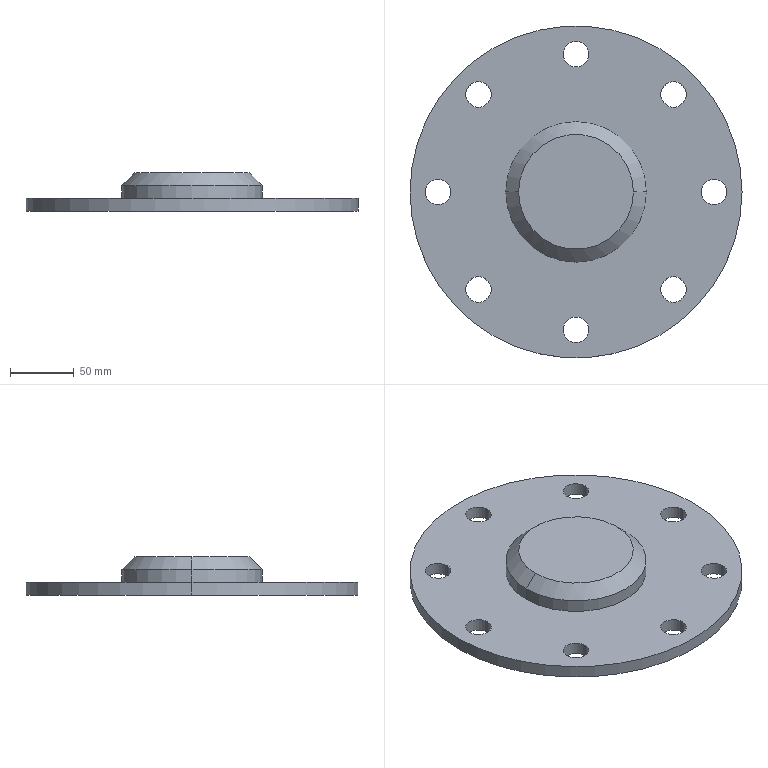Part | SolidWorks | features ICE 2, Chamfer 1, Extrusion 1 | 1 solid | 28 faces | box 260 x 260 x 30 mm | volume 552397 mm3 | cylinder 22 | plane 4 | cone 2 | commonest cylinder face diameters 20 x16 90 x2 110 x2 260 x2
STEP:
#1=CARTESIAN_POINT('',(45.,0.,30.));
#2=VERTEX_POINT('',#1);
#3=CARTESIAN_POINT('',(-45.,0.,30.));
#4=VERTEX_POINT('',#3);
#5=CARTESIAN_POINT('',(0.,0.,30.));
#6=DIRECTION('',(0.,0.,1.));
#7=DIRECTION('',(1.,0.,0.));
#8=AXIS2_PLACEMENT_3D('',#5,#6,#7);
#9=CIRCLE('',#8,45.);
#10=EDGE_CURVE('',#2,#4,#9,.T.);
#11=ORIENTED_EDGE('',*,*,#10,.F.);
#12=CARTESIAN_POINT('',(55.,0.,20.));
#13=VERTEX_POINT('',#12);
#14=CARTESIAN_POINT('',(45.,0.,30.));
#15=DIRECTION('',(0.7071,0.,-0.7071));
#16=VECTOR('',#15,1000.);
#17=LINE('',#14,#16);
#18=EDGE_CURVE('',#2,#13,#17,.T.);
#19=ORIENTED_EDGE('',*,*,#18,.T.);
#20=CARTESIAN_POINT('',(-55.,0.,20.));
#21=VERTEX_POINT('',#20);
#22=CARTESIAN_POINT('',(0.,0.,20.));
#23=DIRECTION('',(0.,0.,-1.));
#24=DIRECTION('',(1.,0.,0.));
#25=AXIS2_PLACEMENT_3D('',#22,#23,#24);
#26=CIRCLE('',#25,55.);
#27=EDGE_CURVE('',#21,#13,#26,.T.);
#28=ORIENTED_EDGE('',*,*,#27,.F.);
#29=CARTESIAN_POINT('',(-45.,0.,30.));
#30=DIRECTION('',(-0.7071,0.,-0.7071));
#31=VECTOR('',#30,1000.);
#32=LINE('',#29,#31);
#33=EDGE_CURVE('',#4,#21,#32,.T.);
#34=ORIENTED_EDGE('',*,*,#33,.F.);
#35=EDGE_LOOP('',(#11,#19,#28,#34));
#36=FACE_OUTER_BOUND('',#35,.T.);
#37=CARTESIAN_POINT('',(0.,0.,30.));
#38=DIRECTION('',(0.,0.,-1.));
#39=DIRECTION('',(-1.,0.,0.));
#40=AXIS2_PLACEMENT_3D('',#37,#38,#39);
#41=CONICAL_SURFACE('',#40,45.,0.7854);
#42=ADVANCED_FACE('',(#36),#41,.T.);
#43=CARTESIAN_POINT('',(45.,0.,20.));
#44=VERTEX_POINT('',#43);
#45=CARTESIAN_POINT('',(-45.,0.,20.));
#46=VERTEX_POINT('',#45);
#47=CARTESIAN_POINT('',(0.,0.,20.));
#48=DIRECTION('',(0.,0.,-1.));
#49=DIRECTION('',(-1.,0.,0.));
#50=AXIS2_PLACEMENT_3D('',#47,#48,#49);
#51=CIRCLE('',#50,45.);
#52=EDGE_CURVE('',#44,#46,#51,.T.);
#53=ORIENTED_EDGE('',*,*,#52,.F.);
#54=CARTESIAN_POINT('',(45.,0.,0.));
#55=VERTEX_POINT('',#54);
#56=CARTESIAN_POINT('',(45.,0.,20.));
#57=DIRECTION('',(0.,0.,-1.));
#58=VECTOR('',#57,1000.);
#59=LINE('',#56,#58);
#60=EDGE_CURVE('',#44,#55,#59,.T.);
#61=ORIENTED_EDGE('',*,*,#60,.T.);
#62=CARTESIAN_POINT('',(-45.,0.,0.));
#63=VERTEX_POINT('',#62);
#64=CARTESIAN_POINT('',(0.,0.,0.));
#65=DIRECTION('',(0.,0.,-1.));
#66=DIRECTION('',(-1.,0.,0.));
#67=AXIS2_PLACEMENT_3D('',#64,#65,#66);
#68=CIRCLE('',#67,45.);
#69=EDGE_CURVE('',#55,#63,#68,.T.);
#70=ORIENTED_EDGE('',*,*,#69,.T.);
#71=CARTESIAN_POINT('',(-45.,0.,20.));
#72=DIRECTION('',(0.,0.,-1.));
#73=VECTOR('',#72,1000.);
#74=LINE('',#71,#73);
#75=EDGE_CURVE('',#46,#63,#74,.T.);
#76=ORIENTED_EDGE('',*,*,#75,.F.);
#77=EDGE_LOOP('',(#53,#61,#70,#76));
#78=FACE_OUTER_BOUND('',#77,.T.);
#79=CARTESIAN_POINT('',(0.,0.,20.));
#80=DIRECTION('',(0.,0.,-1.));
#81=DIRECTION('',(-1.,0.,0.));
#82=AXIS2_PLACEMENT_3D('',#79,#80,#81);
#83=CYLINDRICAL_SURFACE('',#82,45.);
#84=ADVANCED_FACE('',(#78),#83,.F.);
#85=ORIENTED_EDGE('',*,*,#27,.T.);
#86=CARTESIAN_POINT('',(55.,0.,10.));
#87=VERTEX_POINT('',#86);
#88=CARTESIAN_POINT('',(55.,0.,30.));
#89=DIRECTION('',(0.,0.,-1.));
#90=VECTOR('',#89,1000.);
#91=LINE('',#88,#90);
#92=EDGE_CURVE('',#13,#87,#91,.T.);
#93=ORIENTED_EDGE('',*,*,#92,.T.);
#94=CARTESIAN_POINT('',(-55.,0.,10.));
#95=VERTEX_POINT('',#94);
#96=CARTESIAN_POINT('',(0.,0.,10.));
#97=DIRECTION('',(0.,0.,1.));
#98=DIRECTION('',(1.,0.,0.));
#99=AXIS2_PLACEMENT_3D('',#96,#97,#98);
#100=CIRCLE('',#99,55.);
#101=EDGE_CURVE('',#87,#95,#100,.T.);
#102=ORIENTED_EDGE('',*,*,#101,.T.);
#103=CARTESIAN_POINT('',(-55.,0.,30.));
#104=DIRECTION('',(0.,0.,-1.));
#105=VECTOR('',#104,1000.);
#106=LINE('',#103,#105);
#107=EDGE_CURVE('',#21,#95,#106,.T.);
#108=ORIENTED_EDGE('',*,*,#107,.F.);
#109=EDGE_LOOP('',(#85,#93,#102,#108));
#110=FACE_OUTER_BOUND('',#109,.T.);
#111=CARTESIAN_POINT('',(0.,0.,30.));
#112=DIRECTION('',(0.,0.,-1.));
#113=DIRECTION('',(-1.,0.,0.));
#114=AXIS2_PLACEMENT_3D('',#111,#112,#113);
#115=CYLINDRICAL_SURFACE('',#114,55.);
#116=ADVANCED_FACE('',(#110),#115,.T.);
#117=CARTESIAN_POINT('',(-86.368,76.368,10.));
#118=VERTEX_POINT('',#117);
#119=CARTESIAN_POINT('',(-66.368,76.368,10.));
#120=VERTEX_POINT('',#119);
#121=CARTESIAN_POINT('',(-76.368,76.368,10.));
#122=DIRECTION('',(0.,0.,1.));
#123=DIRECTION('',(1.,0.,0.));
#124=AXIS2_PLACEMENT_3D('',#121,#122,#123);
#125=CIRCLE('',#124,10.);
#126=EDGE_CURVE('',#118,#120,#125,.T.);
#127=ORIENTED_EDGE('',*,*,#126,.T.);
#128=CARTESIAN_POINT('',(-66.368,76.368,0.));
#129=VERTEX_POINT('',#128);
#130=CARTESIAN_POINT('',(-66.368,76.368,10.));
#131=DIRECTION('',(0.,0.,-1.));
#132=VECTOR('',#131,1000.);
#133=LINE('',#130,#132);
#134=EDGE_CURVE('',#120,#129,#133,.T.);
#135=ORIENTED_EDGE('',*,*,#134,.T.);
#136=CARTESIAN_POINT('',(-86.368,76.368,0.));
#137=VERTEX_POINT('',#136);
#138=CARTESIAN_POINT('',(-76.368,76.368,0.));
#139=DIRECTION('',(0.,0.,1.));
#140=DIRECTION('',(1.,0.,0.));
#141=AXIS2_PLACEMENT_3D('',#138,#139,#140);
#142=CIRCLE('',#141,10.);
#143=EDGE_CURVE('',#137,#129,#142,.T.);
#144=ORIENTED_EDGE('',*,*,#143,.F.);
#145=CARTESIAN_POINT('',(-86.368,76.368,10.));
#146=DIRECTION('',(0.,0.,-1.));
#147=VECTOR('',#146,1000.);
#148=LINE('',#145,#147);
#149=EDGE_CURVE('',#118,#137,#148,.T.);
#150=ORIENTED_EDGE('',*,*,#149,.F.);
#151=EDGE_LOOP('',(#127,#135,#144,#150));
#152=FACE_OUTER_BOUND('',#151,.T.);
#153=CARTESIAN_POINT('',(-76.368,76.368,10.));
#154=DIRECTION('',(0.,0.,-1.));
#155=DIRECTION('',(-1.,0.,0.));
#156=AXIS2_PLACEMENT_3D('',#153,#154,#155);
#157=CYLINDRICAL_SURFACE('',#156,10.);
#158=ADVANCED_FACE('',(#152),#157,.F.);
#159=CARTESIAN_POINT('',(-118.,0.,10.));
#160=VERTEX_POINT('',#159);
#161=CARTESIAN_POINT('',(-98.,0.,10.));
#162=VERTEX_POINT('',#161);
#163=CARTESIAN_POINT('',(-108.,0.,10.));
#164=DIRECTION('',(0.,0.,1.));
#165=DIRECTION('',(1.,0.,0.));
#166=AXIS2_PLACEMENT_3D('',#163,#164,#165);
#167=CIRCLE('',#166,10.);
#168=EDGE_CURVE('',#160,#162,#167,.T.);
#169=ORIENTED_EDGE('',*,*,#168,.T.);
#170=CARTESIAN_POINT('',(-98.,0.,0.));
#171=VERTEX_POINT('',#170);
#172=CARTESIAN_POINT('',(-98.,0.,10.));
#173=DIRECTION('',(0.,0.,-1.));
#174=VECTOR('',#173,1000.);
#175=LINE('',#172,#174);
#176=EDGE_CURVE('',#162,#171,#175,.T.);
#177=ORIENTED_EDGE('',*,*,#176,.T.);
#178=CARTESIAN_POINT('',(-118.,0.,0.));
#179=VERTEX_POINT('',#178);
#180=CARTESIAN_POINT('',(-108.,0.,0.));
#181=DIRECTION('',(0.,0.,1.));
#182=DIRECTION('',(1.,0.,0.));
#183=AXIS2_PLACEMENT_3D('',#180,#181,#182);
#184=CIRCLE('',#183,10.);
#185=EDGE_CURVE('',#179,#171,#184,.T.);
#186=ORIENTED_EDGE('',*,*,#185,.F.);
#187=CARTESIAN_POINT('',(-118.,0.,10.));
#188=DIRECTION('',(0.,0.,-1.));
#189=VECTOR('',#188,1000.);
#190=LINE('',#187,#189);
#191=EDGE_CURVE('',#160,#179,#190,.T.);
#192=ORIENTED_EDGE('',*,*,#191,.F.);
#193=EDGE_LOOP('',(#169,#177,#186,#192));
#194=FACE_OUTER_BOUND('',#193,.T.);
#195=CARTESIAN_POINT('',(-108.,0.,10.));
#196=DIRECTION('',(0.,0.,-1.));
#197=DIRECTION('',(-1.,0.,0.));
#198=AXIS2_PLACEMENT_3D('',#195,#196,#197);
#199=CYLINDRICAL_SURFACE('',#198,10.);
#200=ADVANCED_FACE('',(#194),#199,.F.);
#201=CARTESIAN_POINT('',(-86.368,-76.368,10.));
#202=VERTEX_POINT('',#201);
#203=CARTESIAN_POINT('',(-66.368,-76.368,10.));
#204=VERTEX_POINT('',#203);
#205=CARTESIAN_POINT('',(-76.368,-76.368,10.));
#206=DIRECTION('',(0.,0.,1.));
#207=DIRECTION('',(1.,0.,0.));
#208=AXIS2_PLACEMENT_3D('',#205,#206,#207);
#209=CIRCLE('',#208,10.);
#210=EDGE_CURVE('',#202,#204,#209,.T.);
#211=ORIENTED_EDGE('',*,*,#210,.T.);
#212=CARTESIAN_POINT('',(-66.368,-76.368,0.));
#213=VERTEX_POINT('',#212);
#214=CARTESIAN_POINT('',(-66.368,-76.368,10.));
#215=DIRECTION('',(0.,0.,-1.));
#216=VECTOR('',#215,1000.);
#217=LINE('',#214,#216);
#218=EDGE_CURVE('',#204,#213,#217,.T.);
#219=ORIENTED_EDGE('',*,*,#218,.T.);
#220=CARTESIAN_POINT('',(-86.368,-76.368,0.));
#221=VERTEX_POINT('',#220);
#222=CARTESIAN_POINT('',(-76.368,-76.368,0.));
#223=DIRECTION('',(0.,0.,1.));
#224=DIRECTION('',(1.,0.,0.));
#225=AXIS2_PLACEMENT_3D('',#222,#223,#224);
#226=CIRCLE('',#225,10.);
#227=EDGE_CURVE('',#221,#213,#226,.T.);
#228=ORIENTED_EDGE('',*,*,#227,.F.);
#229=CARTESIAN_POINT('',(-86.368,-76.368,10.));
#230=DIRECTION('',(0.,0.,-1.));
#231=VECTOR('',#230,1000.);
#232=LINE('',#229,#231);
#233=EDGE_CURVE('',#202,#221,#232,.T.);
#234=ORIENTED_EDGE('',*,*,#233,.F.);
#235=EDGE_LOOP('',(#211,#219,#228,#234));
#236=FACE_OUTER_BOUND('',#235,.T.);
#237=CARTESIAN_POINT('',(-76.368,-76.368,10.));
#238=DIRECTION('',(0.,0.,-1.));
#239=DIRECTION('',(-1.,0.,0.));
#240=AXIS2_PLACEMENT_3D('',#237,#238,#239);
#241=CYLINDRICAL_SURFACE('',#240,10.);
#242=ADVANCED_FACE('',(#236),#241,.F.);
#243=CARTESIAN_POINT('',(-10.,-108.,10.));
#244=VERTEX_POINT('',#243);
#245=CARTESIAN_POINT('',(10.,-108.,10.));
#246=VERTEX_POINT('',#245);
#247=CARTESIAN_POINT('',(0.,-108.,10.));
#248=DIRECTION('',(0.,0.,1.));
#249=DIRECTION('',(1.,0.,0.));
#250=AXIS2_PLACEMENT_3D('',#247,#248,#249);
#251=CIRCLE('',#250,10.);
#252=EDGE_CURVE('',#244,#246,#251,.T.);
#253=ORIENTED_EDGE('',*,*,#252,.T.);
#254=CARTESIAN_POINT('',(10.,-108.,0.));
#255=VERTEX_POINT('',#254);
#256=CARTESIAN_POINT('',(10.,-108.,10.));
#257=DIRECTION('',(0.,0.,-1.));
#258=VECTOR('',#257,1000.);
#259=LINE('',#256,#258);
#260=EDGE_CURVE('',#246,#255,#259,.T.);
#261=ORIENTED_EDGE('',*,*,#260,.T.);
#262=CARTESIAN_POINT('',(-10.,-108.,0.));
#263=VERTEX_POINT('',#262);
#264=CARTESIAN_POINT('',(0.,-108.,0.));
#265=DIRECTION('',(0.,0.,1.));
#266=DIRECTION('',(1.,0.,0.));
#267=AXIS2_PLACEMENT_3D('',#264,#265,#266);
#268=CIRCLE('',#267,10.);
#269=EDGE_CURVE('',#263,#255,#268,.T.);
#270=ORIENTED_EDGE('',*,*,#269,.F.);
#271=CARTESIAN_POINT('',(-10.,-108.,10.));
#272=DIRECTION('',(0.,0.,-1.));
#273=VECTOR('',#272,1000.);
#274=LINE('',#271,#273);
#275=EDGE_CURVE('',#244,#263,#274,.T.);
#276=ORIENTED_EDGE('',*,*,#275,.F.);
#277=EDGE_LOOP('',(#253,#261,#270,#276));
#278=FACE_OUTER_BOUND('',#277,.T.);
#279=CARTESIAN_POINT('',(0.,-108.,10.));
#280=DIRECTION('',(0.,0.,-1.));
#281=DIRECTION('',(-1.,0.,0.));
#282=AXIS2_PLACEMENT_3D('',#279,#280,#281);
#283=CYLINDRICAL_SURFACE('',#282,10.);
#284=ADVANCED_FACE('',(#278),#283,.F.);
#285=CARTESIAN_POINT('',(66.368,-76.368,10.));
#286=VERTEX_POINT('',#285);
#287=CARTESIAN_POINT('',(86.368,-76.368,10.));
#288=VERTEX_POINT('',#287);
#289=CARTESIAN_POINT('',(76.368,-76.368,10.));
#290=DIRECTION('',(0.,0.,1.));
#291=DIRECTION('',(1.,0.,0.));
#292=AXIS2_PLACEMENT_3D('',#289,#290,#291);
#293=CIRCLE('',#292,10.);
#294=EDGE_CURVE('',#286,#288,#293,.T.);
#295=ORIENTED_EDGE('',*,*,#294,.T.);
#296=CARTESIAN_POINT('',(86.368,-76.368,0.));
#297=VERTEX_POINT('',#296);
#298=CARTESIAN_POINT('',(86.368,-76.368,10.));
#299=DIRECTION('',(0.,0.,-1.));
#300=VECTOR('',#299,1000.);
#301=LINE('',#298,#300);
#302=EDGE_CURVE('',#288,#297,#301,.T.);
#303=ORIENTED_EDGE('',*,*,#302,.T.);
#304=CARTESIAN_POINT('',(66.368,-76.368,0.));
#305=VERTEX_POINT('',#304);
#306=CARTESIAN_POINT('',(76.368,-76.368,0.));
#307=DIRECTION('',(0.,0.,1.));
#308=DIRECTION('',(1.,0.,0.));
#309=AXIS2_PLACEMENT_3D('',#306,#307,#308);
#310=CIRCLE('',#309,10.);
#311=EDGE_CURVE('',#305,#297,#310,.T.);
#312=ORIENTED_EDGE('',*,*,#311,.F.);
#313=CARTESIAN_POINT('',(66.368,-76.368,10.));
#314=DIRECTION('',(0.,0.,-1.));
#315=VECTOR('',#314,1000.);
#316=LINE('',#313,#315);
#317=EDGE_CURVE('',#286,#305,#316,.T.);
#318=ORIENTED_EDGE('',*,*,#317,.F.);
#319=EDGE_LOOP('',(#295,#303,#312,#318));
#320=FACE_OUTER_BOUND('',#319,.T.);
#321=CARTESIAN_POINT('',(76.368,-76.368,10.));
#322=DIRECTION('',(0.,0.,-1.));
#323=DIRECTION('',(-1.,0.,0.));
#324=AXIS2_PLACEMENT_3D('',#321,#322,#323);
#325=CYLINDRICAL_SURFACE('',#324,10.);
#326=ADVANCED_FACE('',(#320),#325,.F.);
#327=CARTESIAN_POINT('',(98.,0.,10.));
#328=VERTEX_POINT('',#327);
#329=CARTESIAN_POINT('',(118.,0.,10.));
#330=VERTEX_POINT('',#329);
#331=CARTESIAN_POINT('',(108.,0.,10.));
#332=DIRECTION('',(0.,0.,1.));
#333=DIRECTION('',(1.,0.,0.));
#334=AXIS2_PLACEMENT_3D('',#331,#332,#333);
#335=CIRCLE('',#334,10.);
#336=EDGE_CURVE('',#328,#330,#335,.T.);
#337=ORIENTED_EDGE('',*,*,#336,.T.);
#338=CARTESIAN_POINT('',(118.,0.,0.));
#339=VERTEX_POINT('',#338);
#340=CARTESIAN_POINT('',(118.,0.,10.));
#341=DIRECTION('',(0.,0.,-1.));
#342=VECTOR('',#341,1000.);
#343=LINE('',#340,#342);
#344=EDGE_CURVE('',#330,#339,#343,.T.);
#345=ORIENTED_EDGE('',*,*,#344,.T.);
#346=CARTESIAN_POINT('',(98.,0.,0.));
#347=VERTEX_POINT('',#346);
#348=CARTESIAN_POINT('',(108.,0.,0.));
#349=DIRECTION('',(0.,0.,1.));
#350=DIRECTION('',(1.,0.,0.));
#351=AXIS2_PLACEMENT_3D('',#348,#349,#350);
#352=CIRCLE('',#351,10.);
#353=EDGE_CURVE('',#347,#339,#352,.T.);
#354=ORIENTED_EDGE('',*,*,#353,.F.);
#355=CARTESIAN_POINT('',(98.,0.,10.));
#356=DIRECTION('',(0.,0.,-1.));
#357=VECTOR('',#356,1000.);
#358=LINE('',#355,#357);
#359=EDGE_CURVE('',#328,#347,#358,.T.);
#360=ORIENTED_EDGE('',*,*,#359,.F.);
#361=EDGE_LOOP('',(#337,#345,#354,#360));
#362=FACE_OUTER_BOUND('',#361,.T.);
#363=CARTESIAN_POINT('',(108.,0.,10.));
#364=DIRECTION('',(0.,0.,-1.));
#365=DIRECTION('',(-1.,0.,0.));
#366=AXIS2_PLACEMENT_3D('',#363,#364,#365);
#367=CYLINDRICAL_SURFACE('',#366,10.);
#368=ADVANCED_FACE('',(#362),#367,.F.);
#369=CARTESIAN_POINT('',(66.368,76.368,10.));
#370=VERTEX_POINT('',#369);
#371=CARTESIAN_POINT('',(86.368,76.368,10.));
#372=VERTEX_POINT('',#371);
#373=CARTESIAN_POINT('',(76.368,76.368,10.));
#374=DIRECTION('',(0.,0.,1.));
#375=DIRECTION('',(1.,0.,0.));
#376=AXIS2_PLACEMENT_3D('',#373,#374,#375);
#377=CIRCLE('',#376,10.);
#378=EDGE_CURVE('',#370,#372,#377,.T.);
#379=ORIENTED_EDGE('',*,*,#378,.T.);
#380=CARTESIAN_POINT('',(86.368,76.368,0.));
#381=VERTEX_POINT('',#380);
#382=CARTESIAN_POINT('',(86.368,76.368,10.));
#383=DIRECTION('',(0.,0.,-1.));
#384=VECTOR('',#383,1000.);
#385=LINE('',#382,#384);
#386=EDGE_CURVE('',#372,#381,#385,.T.);
#387=ORIENTED_EDGE('',*,*,#386,.T.);
#388=CARTESIAN_POINT('',(66.368,76.368,0.));
#389=VERTEX_POINT('',#388);
#390=CARTESIAN_POINT('',(76.368,76.368,0.));
#391=DIRECTION('',(0.,0.,1.));
#392=DIRECTION('',(1.,0.,0.));
#393=AXIS2_PLACEMENT_3D('',#390,#391,#392);
#394=CIRCLE('',#393,10.);
#395=EDGE_CURVE('',#389,#381,#394,.T.);
#396=ORIENTED_EDGE('',*,*,#395,.F.);
#397=CARTESIAN_POINT('',(66.368,76.368,10.));
#398=DIRECTION('',(0.,0.,-1.));
#399=VECTOR('',#398,1000.);
#400=LINE('',#397,#399);
#401=EDGE_CURVE('',#370,#389,#400,.T.);
#402=ORIENTED_EDGE('',*,*,#401,.F.);
#403=EDGE_LOOP('',(#379,#387,#396,#402));
#404=FACE_OUTER_BOUND('',#403,.T.);
#405=CARTESIAN_POINT('',(76.368,76.368,10.));
#406=DIRECTION('',(0.,0.,-1.));
#407=DIRECTION('',(-1.,0.,0.));
#408=AXIS2_PLACEMENT_3D('',#405,#406,#407);
#409=CYLINDRICAL_SURFACE('',#408,10.);
#410=ADVANCED_FACE('',(#404),#409,.F.);
#411=CARTESIAN_POINT('',(-10.,108.,10.));
#412=VERTEX_POINT('',#411);
#413=CARTESIAN_POINT('',(10.,108.,10.));
#414=VERTEX_POINT('',#413);
#415=CARTESIAN_POINT('',(0.,108.,10.));
#416=DIRECTION('',(0.,0.,1.));
#417=DIRECTION('',(1.,0.,0.));
#418=AXIS2_PLACEMENT_3D('',#415,#416,#417);
#419=CIRCLE('',#418,10.);
#420=EDGE_CURVE('',#412,#414,#419,.T.);
#421=ORIENTED_EDGE('',*,*,#420,.T.);
#422=CARTESIAN_POINT('',(10.,108.,0.));
#423=VERTEX_POINT('',#422);
#424=CARTESIAN_POINT('',(10.,108.,10.));
#425=DIRECTION('',(0.,0.,-1.));
#426=VECTOR('',#425,1000.);
#427=LINE('',#424,#426);
#428=EDGE_CURVE('',#414,#423,#427,.T.);
#429=ORIENTED_EDGE('',*,*,#428,.T.);
#430=CARTESIAN_POINT('',(-10.,108.,0.));
#431=VERTEX_POINT('',#430);
#432=CARTESIAN_POINT('',(0.,108.,0.));
#433=DIRECTION('',(0.,0.,1.));
#434=DIRECTION('',(1.,0.,0.));
#435=AXIS2_PLACEMENT_3D('',#432,#433,#434);
#436=CIRCLE('',#435,10.);
#437=EDGE_CURVE('',#431,#423,#436,.T.);
#438=ORIENTED_EDGE('',*,*,#437,.F.);
#439=CARTESIAN_POINT('',(-10.,108.,10.));
#440=DIRECTION('',(0.,0.,-1.));
#441=VECTOR('',#440,1000.);
#442=LINE('',#439,#441);
#443=EDGE_CURVE('',#412,#431,#442,.T.);
#444=ORIENTED_EDGE('',*,*,#443,.F.);
#445=EDGE_LOOP('',(#421,#429,#438,#444));
#446=FACE_OUTER_BOUND('',#445,.T.);
#447=CARTESIAN_POINT('',(0.,108.,10.));
#448=DIRECTION('',(0.,0.,-1.));
#449=DIRECTION('',(-1.,0.,0.));
#450=AXIS2_PLACEMENT_3D('',#447,#448,#449);
#451=CYLINDRICAL_SURFACE('',#450,10.);
#452=ADVANCED_FACE('',(#446),#451,.F.);
#453=CARTESIAN_POINT('',(130.,0.,10.));
#454=VERTEX_POINT('',#453);
#455=CARTESIAN_POINT('',(-130.,0.,10.));
#456=VERTEX_POINT('',#455);
#457=CARTESIAN_POINT('',(0.,0.,10.));
#458=DIRECTION('',(0.,0.,1.));
#459=DIRECTION('',(1.,0.,0.));
#460=AXIS2_PLACEMENT_3D('',#457,#458,#459);
#461=CIRCLE('',#460,130.);
#462=EDGE_CURVE('',#454,#456,#461,.T.);
#463=ORIENTED_EDGE('',*,*,#462,.F.);
#464=CARTESIAN_POINT('',(130.,0.,0.));
#465=VERTEX_POINT('',#464);
#466=CARTESIAN_POINT('',(130.,0.,10.));
#467=DIRECTION('',(0.,0.,-1.));
#468=VECTOR('',#467,1000.);
#469=LINE('',#466,#468);
#470=EDGE_CURVE('',#454,#465,#469,.T.);
#471=ORIENTED_EDGE('',*,*,#470,.T.);
#472=CARTESIAN_POINT('',(-130.,0.,0.));
#473=VERTEX_POINT('',#472);
#474=CARTESIAN_POINT('',(0.,0.,0.));
#475=DIRECTION('',(0.,0.,1.));
#476=DIRECTION('',(1.,0.,0.));
#477=AXIS2_PLACEMENT_3D('',#474,#475,#476);
#478=CIRCLE('',#477,130.);
#479=EDGE_CURVE('',#465,#473,#478,.T.);
#480=ORIENTED_EDGE('',*,*,#479,.T.);
#481=CARTESIAN_POINT('',(-130.,0.,10.));
#482=DIRECTION('',(0.,0.,-1.));
#483=VECTOR('',#482,1000.);
#484=LINE('',#481,#483);
#485=EDGE_CURVE('',#456,#473,#484,.T.);
#486=ORIENTED_EDGE('',*,*,#485,.F.);
#487=EDGE_LOOP('',(#463,#471,#480,#486));
#488=FACE_OUTER_BOUND('',#487,.T.);
#489=CARTESIAN_POINT('',(0.,0.,10.));
#490=DIRECTION('',(0.,0.,-1.));
#491=DIRECTION('',(-1.,0.,0.));
#492=AXIS2_PLACEMENT_3D('',#489,#490,#491);
#493=CYLINDRICAL_SURFACE('',#492,130.);
#494=ADVANCED_FACE('',(#488),#493,.T.);
#495=CARTESIAN_POINT('',(0.,0.,10.));
#496=DIRECTION('',(0.,0.,1.));
#497=DIRECTION('',(1.,0.,0.));
#498=AXIS2_PLACEMENT_3D('',#495,#496,#497);
#499=CIRCLE('',#498,55.);
#500=EDGE_CURVE('',#95,#87,#499,.T.);
#501=ORIENTED_EDGE('',*,*,#500,.F.);
#502=ORIENTED_EDGE('',*,*,#101,.F.);
#503=EDGE_LOOP('',(#501,#502));
#504=FACE_BOUND('',#503,.T.);
#505=ORIENTED_EDGE('',*,*,#168,.F.);
#506=CARTESIAN_POINT('',(-108.,0.,10.));
#507=DIRECTION('',(0.,0.,1.));
#508=DIRECTION('',(1.,0.,0.));
#509=AXIS2_PLACEMENT_3D('',#506,#507,#508);
#510=CIRCLE('',#509,10.);
#511=EDGE_CURVE('',#162,#160,#510,.T.);
#512=ORIENTED_EDGE('',*,*,#511,.F.);
#513=EDGE_LOOP('',(#505,#512));
#514=FACE_BOUND('',#513,.T.);
#515=ORIENTED_EDGE('',*,*,#252,.F.);
#516=CARTESIAN_POINT('',(0.,-108.,10.));
#517=DIRECTION('',(0.,0.,1.));
#518=DIRECTION('',(1.,0.,0.));
#519=AXIS2_PLACEMENT_3D('',#516,#517,#518);
#520=CIRCLE('',#519,10.);
#521=EDGE_CURVE('',#246,#244,#520,.T.);
#522=ORIENTED_EDGE('',*,*,#521,.F.);
#523=EDGE_LOOP('',(#515,#522));
#524=FACE_BOUND('',#523,.T.);
#525=ORIENTED_EDGE('',*,*,#336,.F.);
#526=CARTESIAN_POINT('',(108.,0.,10.));
#527=DIRECTION('',(0.,0.,1.));
#528=DIRECTION('',(1.,0.,0.));
#529=AXIS2_PLACEMENT_3D('',#526,#527,#528);
#530=CIRCLE('',#529,10.);
#531=EDGE_CURVE('',#330,#328,#530,.T.);
#532=ORIENTED_EDGE('',*,*,#531,.F.);
#533=EDGE_LOOP('',(#525,#532));
#534=FACE_BOUND('',#533,.T.);
#535=ORIENTED_EDGE('',*,*,#420,.F.);
#536=CARTESIAN_POINT('',(0.,108.,10.));
#537=DIRECTION('',(0.,0.,1.));
#538=DIRECTION('',(1.,0.,0.));
#539=AXIS2_PLACEMENT_3D('',#536,#537,#538);
#540=CIRCLE('',#539,10.);
#541=EDGE_CURVE('',#414,#412,#540,.T.);
#542=ORIENTED_EDGE('',*,*,#541,.F.);
#543=EDGE_LOOP('',(#535,#542));
#544=FACE_BOUND('',#543,.T.);
#545=CARTESIAN_POINT('',(0.,0.,10.));
#546=DIRECTION('',(0.,0.,1.));
#547=DIRECTION('',(1.,0.,0.));
#548=AXIS2_PLACEMENT_3D('',#545,#546,#547);
#549=CIRCLE('',#548,130.);
#550=EDGE_CURVE('',#456,#454,#549,.T.);
#551=ORIENTED_EDGE('',*,*,#550,.T.);
#552=ORIENTED_EDGE('',*,*,#462,.T.);
#553=EDGE_LOOP('',(#551,#552));
#554=FACE_OUTER_BOUND('',#553,.T.);
#555=ORIENTED_EDGE('',*,*,#378,.F.);
#556=CARTESIAN_POINT('',(76.368,76.368,10.));
#557=DIRECTION('',(0.,0.,1.));
#558=DIRECTION('',(1.,0.,0.));
#559=AXIS2_PLACEMENT_3D('',#556,#557,#558);
#560=CIRCLE('',#559,10.);
#561=EDGE_CURVE('',#372,#370,#560,.T.);
#562=ORIENTED_EDGE('',*,*,#561,.F.);
#563=EDGE_LOOP('',(#555,#562));
#564=FACE_BOUND('',#563,.T.);
#565=ORIENTED_EDGE('',*,*,#294,.F.);
#566=CARTESIAN_POINT('',(76.368,-76.368,10.));
#567=DIRECTION('',(0.,0.,1.));
#568=DIRECTION('',(1.,0.,0.));
#569=AXIS2_PLACEMENT_3D('',#566,#567,#568);
#570=CIRCLE('',#569,10.);
#571=EDGE_CURVE('',#288,#286,#570,.T.);
#572=ORIENTED_EDGE('',*,*,#571,.F.);
#573=EDGE_LOOP('',(#565,#572));
#574=FACE_BOUND('',#573,.T.);
#575=ORIENTED_EDGE('',*,*,#210,.F.);
#576=CARTESIAN_POINT('',(-76.368,-76.368,10.));
#577=DIRECTION('',(0.,0.,1.));
#578=DIRECTION('',(1.,0.,0.));
#579=AXIS2_PLACEMENT_3D('',#576,#577,#578);
#580=CIRCLE('',#579,10.);
#581=EDGE_CURVE('',#204,#202,#580,.T.);
#582=ORIENTED_EDGE('',*,*,#581,.F.);
#583=EDGE_LOOP('',(#575,#582));
#584=FACE_BOUND('',#583,.T.);
#585=ORIENTED_EDGE('',*,*,#126,.F.);
#586=CARTESIAN_POINT('',(-76.368,76.368,10.));
#587=DIRECTION('',(0.,0.,1.));
#588=DIRECTION('',(1.,0.,0.));
#589=AXIS2_PLACEMENT_3D('',#586,#587,#588);
#590=CIRCLE('',#589,10.);
#591=EDGE_CURVE('',#120,#118,#590,.T.);
#592=ORIENTED_EDGE('',*,*,#591,.F.);
#593=EDGE_LOOP('',(#585,#592));
#594=FACE_BOUND('',#593,.T.);
#595=CARTESIAN_POINT('',(0.,0.,10.));
#596=DIRECTION('',(0.,0.,1.));
#597=DIRECTION('',(1.,0.,0.));
#598=AXIS2_PLACEMENT_3D('',#595,#596,#597);
#599=PLANE('',#598);
#600=ADVANCED_FACE('',(#504,#514,#524,#534,#544,#554,#564,#574,#584,#594),#599,.T.);
#601=CARTESIAN_POINT('',(0.,0.,0.));
#602=DIRECTION('',(0.,0.,-1.));
#603=DIRECTION('',(-1.,0.,0.));
#604=AXIS2_PLACEMENT_3D('',#601,#602,#603);
#605=CIRCLE('',#604,45.);
#606=EDGE_CURVE('',#63,#55,#605,.T.);
#607=ORIENTED_EDGE('',*,*,#606,.F.);
#608=ORIENTED_EDGE('',*,*,#69,.F.);
#609=EDGE_LOOP('',(#607,#608));
#610=FACE_BOUND('',#609,.T.);
#611=CARTESIAN_POINT('',(0.,0.,0.));
#612=DIRECTION('',(0.,0.,1.));
#613=DIRECTION('',(1.,0.,0.));
#614=AXIS2_PLACEMENT_3D('',#611,#612,#613);
#615=CIRCLE('',#614,130.);
#616=EDGE_CURVE('',#473,#465,#615,.T.);
#617=ORIENTED_EDGE('',*,*,#616,.F.);
#618=ORIENTED_EDGE('',*,*,#479,.F.);
#619=EDGE_LOOP('',(#617,#618));
#620=FACE_OUTER_BOUND('',#619,.T.);
#621=ORIENTED_EDGE('',*,*,#437,.T.);
#622=CARTESIAN_POINT('',(0.,108.,0.));
#623=DIRECTION('',(0.,0.,1.));
#624=DIRECTION('',(1.,0.,0.));
#625=AXIS2_PLACEMENT_3D('',#622,#623,#624);
#626=CIRCLE('',#625,10.);
#627=EDGE_CURVE('',#423,#431,#626,.T.);
#628=ORIENTED_EDGE('',*,*,#627,.T.);
#629=EDGE_LOOP('',(#621,#628));
#630=FACE_BOUND('',#629,.T.);
#631=ORIENTED_EDGE('',*,*,#395,.T.);
#632=CARTESIAN_POINT('',(76.368,76.368,0.));
#633=DIRECTION('',(0.,0.,1.));
#634=DIRECTION('',(1.,0.,0.));
#635=AXIS2_PLACEMENT_3D('',#632,#633,#634);
#636=CIRCLE('',#635,10.);
#637=EDGE_CURVE('',#381,#389,#636,.T.);
#638=ORIENTED_EDGE('',*,*,#637,.T.);
#639=EDGE_LOOP('',(#631,#638));
#640=FACE_BOUND('',#639,.T.);
#641=ORIENTED_EDGE('',*,*,#353,.T.);
#642=CARTESIAN_POINT('',(108.,0.,0.));
#643=DIRECTION('',(0.,0.,1.));
#644=DIRECTION('',(1.,0.,0.));
#645=AXIS2_PLACEMENT_3D('',#642,#643,#644);
#646=CIRCLE('',#645,10.);
#647=EDGE_CURVE('',#339,#347,#646,.T.);
#648=ORIENTED_EDGE('',*,*,#647,.T.);
#649=EDGE_LOOP('',(#641,#648));
#650=FACE_BOUND('',#649,.T.);
#651=ORIENTED_EDGE('',*,*,#311,.T.);
#652=CARTESIAN_POINT('',(76.368,-76.368,0.));
#653=DIRECTION('',(0.,0.,1.));
#654=DIRECTION('',(1.,0.,0.));
#655=AXIS2_PLACEMENT_3D('',#652,#653,#654);
#656=CIRCLE('',#655,10.);
#657=EDGE_CURVE('',#297,#305,#656,.T.);
#658=ORIENTED_EDGE('',*,*,#657,.T.);
#659=EDGE_LOOP('',(#651,#658));
#660=FACE_BOUND('',#659,.T.);
#661=ORIENTED_EDGE('',*,*,#269,.T.);
#662=CARTESIAN_POINT('',(0.,-108.,0.));
#663=DIRECTION('',(0.,0.,1.));
#664=DIRECTION('',(1.,0.,0.));
#665=AXIS2_PLACEMENT_3D('',#662,#663,#664);
#666=CIRCLE('',#665,10.);
#667=EDGE_CURVE('',#255,#263,#666,.T.);
#668=ORIENTED_EDGE('',*,*,#667,.T.);
#669=EDGE_LOOP('',(#661,#668));
#670=FACE_BOUND('',#669,.T.);
#671=ORIENTED_EDGE('',*,*,#227,.T.);
#672=CARTESIAN_POINT('',(-76.368,-76.368,0.));
#673=DIRECTION('',(0.,0.,1.));
#674=DIRECTION('',(1.,0.,0.));
#675=AXIS2_PLACEMENT_3D('',#672,#673,#674);
#676=CIRCLE('',#675,10.);
#677=EDGE_CURVE('',#213,#221,#676,.T.);
#678=ORIENTED_EDGE('',*,*,#677,.T.);
#679=EDGE_LOOP('',(#671,#678));
#680=FACE_BOUND('',#679,.T.);
#681=ORIENTED_EDGE('',*,*,#185,.T.);
#682=CARTESIAN_POINT('',(-108.,0.,0.));
#683=DIRECTION('',(0.,0.,1.));
#684=DIRECTION('',(1.,0.,0.));
#685=AXIS2_PLACEMENT_3D('',#682,#683,#684);
#686=CIRCLE('',#685,10.);
#687=EDGE_CURVE('',#171,#179,#686,.T.);
#688=ORIENTED_EDGE('',*,*,#687,.T.);
#689=EDGE_LOOP('',(#681,#688));
#690=FACE_BOUND('',#689,.T.);
#691=ORIENTED_EDGE('',*,*,#143,.T.);
#692=CARTESIAN_POINT('',(-76.368,76.368,0.));
#693=DIRECTION('',(0.,0.,1.));
#694=DIRECTION('',(1.,0.,0.));
#695=AXIS2_PLACEMENT_3D('',#692,#693,#694);
#696=CIRCLE('',#695,10.);
#697=EDGE_CURVE('',#129,#137,#696,.T.);
#698=ORIENTED_EDGE('',*,*,#697,.T.);
#699=EDGE_LOOP('',(#691,#698));
#700=FACE_BOUND('',#699,.T.);
#701=CARTESIAN_POINT('',(0.,0.,0.));
#702=DIRECTION('',(0.,0.,1.));
#703=DIRECTION('',(1.,0.,0.));
#704=AXIS2_PLACEMENT_3D('',#701,#702,#703);
#705=PLANE('',#704);
#706=ADVANCED_FACE('',(#610,#620,#630,#640,#650,#660,#670,#680,#690,#700),#705,.F.);
#707=ORIENTED_EDGE('',*,*,#470,.F.);
#708=ORIENTED_EDGE('',*,*,#550,.F.);
#709=ORIENTED_EDGE('',*,*,#485,.T.);
#710=ORIENTED_EDGE('',*,*,#616,.T.);
#711=EDGE_LOOP('',(#707,#708,#709,#710));
#712=FACE_OUTER_BOUND('',#711,.T.);
#713=CARTESIAN_POINT('',(0.,0.,10.));
#714=DIRECTION('',(0.,0.,-1.));
#715=DIRECTION('',(-1.,0.,0.));
#716=AXIS2_PLACEMENT_3D('',#713,#714,#715);
#717=CYLINDRICAL_SURFACE('',#716,130.);
#718=ADVANCED_FACE('',(#712),#717,.T.);
#719=ORIENTED_EDGE('',*,*,#428,.F.);
#720=ORIENTED_EDGE('',*,*,#541,.T.);
#721=ORIENTED_EDGE('',*,*,#443,.T.);
#722=ORIENTED_EDGE('',*,*,#627,.F.);
#723=EDGE_LOOP('',(#719,#720,#721,#722));
#724=FACE_OUTER_BOUND('',#723,.T.);
#725=CARTESIAN_POINT('',(0.,108.,10.));
#726=DIRECTION('',(0.,0.,-1.));
#727=DIRECTION('',(-1.,0.,0.));
#728=AXIS2_PLACEMENT_3D('',#725,#726,#727);
#729=CYLINDRICAL_SURFACE('',#728,10.);
#730=ADVANCED_FACE('',(#724),#729,.F.);
#731=ORIENTED_EDGE('',*,*,#386,.F.);
#732=ORIENTED_EDGE('',*,*,#561,.T.);
#733=ORIENTED_EDGE('',*,*,#401,.T.);
#734=ORIENTED_EDGE('',*,*,#637,.F.);
#735=EDGE_LOOP('',(#731,#732,#733,#734));
#736=FACE_OUTER_BOUND('',#735,.T.);
#737=CARTESIAN_POINT('',(76.368,76.368,10.));
#738=DIRECTION('',(0.,0.,-1.));
#739=DIRECTION('',(-1.,0.,0.));
#740=AXIS2_PLACEMENT_3D('',#737,#738,#739);
#741=CYLINDRICAL_SURFACE('',#740,10.);
#742=ADVANCED_FACE('',(#736),#741,.F.);
#743=ORIENTED_EDGE('',*,*,#344,.F.);
#744=ORIENTED_EDGE('',*,*,#531,.T.);
#745=ORIENTED_EDGE('',*,*,#359,.T.);
#746=ORIENTED_EDGE('',*,*,#647,.F.);
#747=EDGE_LOOP('',(#743,#744,#745,#746));
#748=FACE_OUTER_BOUND('',#747,.T.);
#749=CARTESIAN_POINT('',(108.,0.,10.));
#750=DIRECTION('',(0.,0.,-1.));
#751=DIRECTION('',(-1.,0.,0.));
#752=AXIS2_PLACEMENT_3D('',#749,#750,#751);
#753=CYLINDRICAL_SURFACE('',#752,10.);
#754=ADVANCED_FACE('',(#748),#753,.F.);
#755=ORIENTED_EDGE('',*,*,#302,.F.);
#756=ORIENTED_EDGE('',*,*,#571,.T.);
#757=ORIENTED_EDGE('',*,*,#317,.T.);
#758=ORIENTED_EDGE('',*,*,#657,.F.);
#759=EDGE_LOOP('',(#755,#756,#757,#758));
#760=FACE_OUTER_BOUND('',#759,.T.);
#761=CARTESIAN_POINT('',(76.368,-76.368,10.));
#762=DIRECTION('',(0.,0.,-1.));
#763=DIRECTION('',(-1.,0.,0.));
#764=AXIS2_PLACEMENT_3D('',#761,#762,#763);
#765=CYLINDRICAL_SURFACE('',#764,10.);
#766=ADVANCED_FACE('',(#760),#765,.F.);
#767=ORIENTED_EDGE('',*,*,#260,.F.);
#768=ORIENTED_EDGE('',*,*,#521,.T.);
#769=ORIENTED_EDGE('',*,*,#275,.T.);
#770=ORIENTED_EDGE('',*,*,#667,.F.);
#771=EDGE_LOOP('',(#767,#768,#769,#770));
#772=FACE_OUTER_BOUND('',#771,.T.);
#773=CARTESIAN_POINT('',(0.,-108.,10.));
#774=DIRECTION('',(0.,0.,-1.));
#775=DIRECTION('',(-1.,0.,0.));
#776=AXIS2_PLACEMENT_3D('',#773,#774,#775);
#777=CYLINDRICAL_SURFACE('',#776,10.);
#778=ADVANCED_FACE('',(#772),#777,.F.);
#779=ORIENTED_EDGE('',*,*,#218,.F.);
#780=ORIENTED_EDGE('',*,*,#581,.T.);
#781=ORIENTED_EDGE('',*,*,#233,.T.);
#782=ORIENTED_EDGE('',*,*,#677,.F.);
#783=EDGE_LOOP('',(#779,#780,#781,#782));
#784=FACE_OUTER_BOUND('',#783,.T.);
#785=CARTESIAN_POINT('',(-76.368,-76.368,10.));
#786=DIRECTION('',(0.,0.,-1.));
#787=DIRECTION('',(-1.,0.,0.));
#788=AXIS2_PLACEMENT_3D('',#785,#786,#787);
#789=CYLINDRICAL_SURFACE('',#788,10.);
#790=ADVANCED_FACE('',(#784),#789,.F.);
#791=ORIENTED_EDGE('',*,*,#176,.F.);
#792=ORIENTED_EDGE('',*,*,#511,.T.);
#793=ORIENTED_EDGE('',*,*,#191,.T.);
#794=ORIENTED_EDGE('',*,*,#687,.F.);
#795=EDGE_LOOP('',(#791,#792,#793,#794));
#796=FACE_OUTER_BOUND('',#795,.T.);
#797=CARTESIAN_POINT('',(-108.,0.,10.));
#798=DIRECTION('',(0.,0.,-1.));
#799=DIRECTION('',(-1.,0.,0.));
#800=AXIS2_PLACEMENT_3D('',#797,#798,#799);
#801=CYLINDRICAL_SURFACE('',#800,10.);
#802=ADVANCED_FACE('',(#796),#801,.F.);
#803=ORIENTED_EDGE('',*,*,#134,.F.);
#804=ORIENTED_EDGE('',*,*,#591,.T.);
#805=ORIENTED_EDGE('',*,*,#149,.T.);
#806=ORIENTED_EDGE('',*,*,#697,.F.);
#807=EDGE_LOOP('',(#803,#804,#805,#806));
#808=FACE_OUTER_BOUND('',#807,.T.);
#809=CARTESIAN_POINT('',(-76.368,76.368,10.));
#810=DIRECTION('',(0.,0.,-1.));
#811=DIRECTION('',(-1.,0.,0.));
#812=AXIS2_PLACEMENT_3D('',#809,#810,#811);
#813=CYLINDRICAL_SURFACE('',#812,10.);
#814=ADVANCED_FACE('',(#808),#813,.F.);
#815=ORIENTED_EDGE('',*,*,#92,.F.);
#816=CARTESIAN_POINT('',(0.,0.,20.));
#817=DIRECTION('',(0.,0.,-1.));
#818=DIRECTION('',(1.,0.,0.));
#819=AXIS2_PLACEMENT_3D('',#816,#817,#818);
#820=CIRCLE('',#819,55.);
#821=EDGE_CURVE('',#13,#21,#820,.T.);
#822=ORIENTED_EDGE('',*,*,#821,.T.);
#823=ORIENTED_EDGE('',*,*,#107,.T.);
#824=ORIENTED_EDGE('',*,*,#500,.T.);
#825=EDGE_LOOP('',(#815,#822,#823,#824));
#826=FACE_OUTER_BOUND('',#825,.T.);
#827=CARTESIAN_POINT('',(0.,0.,30.));
#828=DIRECTION('',(0.,0.,-1.));
#829=DIRECTION('',(-1.,0.,0.));
#830=AXIS2_PLACEMENT_3D('',#827,#828,#829);
#831=CYLINDRICAL_SURFACE('',#830,55.);
#832=ADVANCED_FACE('',(#826),#831,.T.);
#833=CARTESIAN_POINT('',(0.,0.,30.));
#834=DIRECTION('',(0.,0.,1.));
#835=DIRECTION('',(1.,0.,0.));
#836=AXIS2_PLACEMENT_3D('',#833,#834,#835);
#837=CIRCLE('',#836,45.);
#838=EDGE_CURVE('',#4,#2,#837,.T.);
#839=ORIENTED_EDGE('',*,*,#838,.T.);
#840=ORIENTED_EDGE('',*,*,#10,.T.);
#841=EDGE_LOOP('',(#839,#840));
#842=FACE_OUTER_BOUND('',#841,.T.);
#843=CARTESIAN_POINT('',(0.,0.,30.));
#844=DIRECTION('',(0.,0.,1.));
#845=DIRECTION('',(1.,0.,0.));
#846=AXIS2_PLACEMENT_3D('',#843,#844,#845);
#847=PLANE('',#846);
#848=ADVANCED_FACE('',(#842),#847,.T.);
#849=ORIENTED_EDGE('',*,*,#60,.F.);
#850=CARTESIAN_POINT('',(0.,0.,20.));
#851=DIRECTION('',(0.,0.,-1.));
#852=DIRECTION('',(-1.,0.,0.));
#853=AXIS2_PLACEMENT_3D('',#850,#851,#852);
#854=CIRCLE('',#853,45.);
#855=EDGE_CURVE('',#46,#44,#854,.T.);
#856=ORIENTED_EDGE('',*,*,#855,.F.);
#857=ORIENTED_EDGE('',*,*,#75,.T.);
#858=ORIENTED_EDGE('',*,*,#606,.T.);
#859=EDGE_LOOP('',(#849,#856,#857,#858));
#860=FACE_OUTER_BOUND('',#859,.T.);
#861=CARTESIAN_POINT('',(0.,0.,20.));
#862=DIRECTION('',(0.,0.,-1.));
#863=DIRECTION('',(-1.,0.,0.));
#864=AXIS2_PLACEMENT_3D('',#861,#862,#863);
#865=CYLINDRICAL_SURFACE('',#864,45.);
#866=ADVANCED_FACE('',(#860),#865,.F.);
#867=ORIENTED_EDGE('',*,*,#855,.T.);
#868=ORIENTED_EDGE('',*,*,#52,.T.);
#869=EDGE_LOOP('',(#867,#868));
#870=FACE_OUTER_BOUND('',#869,.T.);
#871=CARTESIAN_POINT('',(0.,0.,20.));
#872=DIRECTION('',(0.,0.,-1.));
#873=DIRECTION('',(-1.,0.,0.));
#874=AXIS2_PLACEMENT_3D('',#871,#872,#873);
#875=PLANE('',#874);
#876=ADVANCED_FACE('',(#870),#875,.T.);
#877=ORIENTED_EDGE('',*,*,#18,.F.);
#878=ORIENTED_EDGE('',*,*,#838,.F.);
#879=ORIENTED_EDGE('',*,*,#33,.T.);
#880=ORIENTED_EDGE('',*,*,#821,.F.);
#881=EDGE_LOOP('',(#877,#878,#879,#880));
#882=FACE_OUTER_BOUND('',#881,.T.);
#883=CARTESIAN_POINT('',(0.,0.,30.));
#884=DIRECTION('',(0.,0.,-1.));
#885=DIRECTION('',(-1.,0.,0.));
#886=AXIS2_PLACEMENT_3D('',#883,#884,#885);
#887=CONICAL_SURFACE('',#886,45.,0.7854);
#888=ADVANCED_FACE('',(#882),#887,.T.);
#889=CLOSED_SHELL('',(#42,#84,#116,#158,#200,#242,#284,#326,#368,#410,#452,#494,#600,#706,#718,#730,#742,#754,#766,#778,#790,#802,#814,#832,#848,#866,#876,#888));
#890=MANIFOLD_SOLID_BREP('',#889);
#891=CARTESIAN_POINT('',(0.,0.,0.));
#892=DIRECTION('',(0.,0.,1.));
#893=DIRECTION('',(1.,0.,0.));
#894=AXIS2_PLACEMENT_3D('',#891,#892,#893);
#895=(LENGTH_UNIT()NAMED_UNIT(*)SI_UNIT(.MILLI.,.METRE.));
#896=UNCERTAINTY_MEASURE_WITH_UNIT(LENGTH_MEASURE(0.00001),#895,'','');
#897=(NAMED_UNIT(*)PLANE_ANGLE_UNIT()SI_UNIT($,.RADIAN.));
#898=(NAMED_UNIT(*)SI_UNIT($,.STERADIAN.)SOLID_ANGLE_UNIT());
#899=(GEOMETRIC_REPRESENTATION_CONTEXT(3)GLOBAL_UNCERTAINTY_ASSIGNED_CONTEXT((#896))GLOBAL_UNIT_ASSIGNED_CONTEXT((#895,#897,#898))REPRESENTATION_CONTEXT('',''));
#900=ADVANCED_BREP_SHAPE_REPRESENTATION('',(#890,#894),#899);